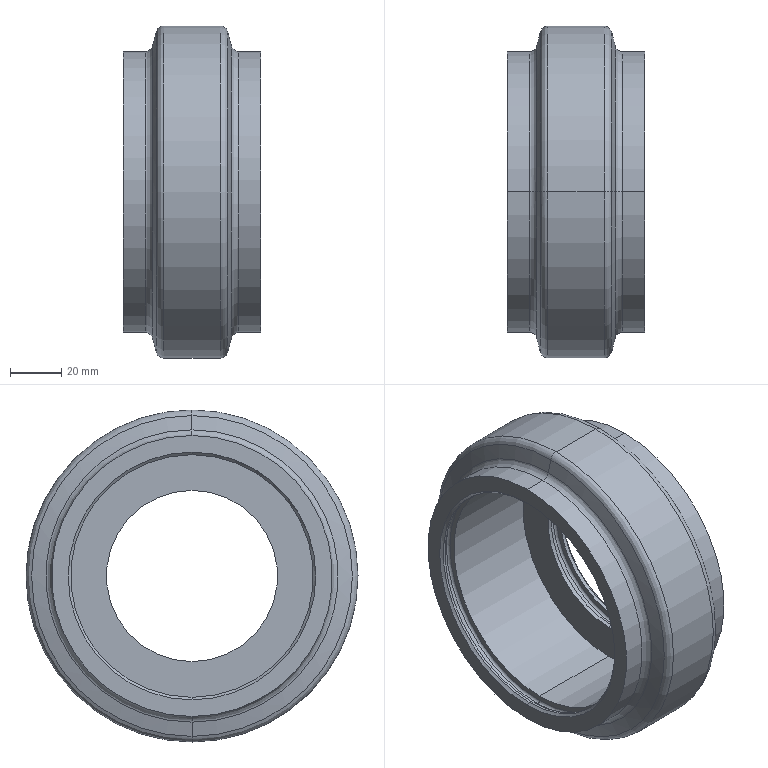Part | SolidWorks | features Chamfer 1, Revolution 1 | 1 solid | 49 faces | box 54 x 130 x 130 mm | volume 264733 mm3 | cylinder 18 | torus 16 | cone 8 | plane 7 | commonest cylinder face diameters 67 x4 95 x4 110 x4 73.2 x2 101.2 x2 130 x2
STEP:
#1=CARTESIAN_POINT('',(-26.,0.,-47.5));
#2=VERTEX_POINT('',#1);
#3=CARTESIAN_POINT('',(-26.,0.,47.5));
#4=VERTEX_POINT('',#3);
#5=CARTESIAN_POINT('',(-26.,0.,0.));
#6=DIRECTION('',(-1.,0.,0.));
#7=DIRECTION('',(0.,0.,1.));
#8=AXIS2_PLACEMENT_3D('',#5,#6,#7);
#9=CIRCLE('',#8,47.5);
#10=EDGE_CURVE('',#2,#4,#9,.T.);
#11=ORIENTED_EDGE('',*,*,#10,.F.);
#12=CARTESIAN_POINT('',(-27.,0.,-48.5));
#13=VERTEX_POINT('',#12);
#14=CARTESIAN_POINT('',(-27.,0.,-48.5));
#15=DIRECTION('',(-0.7071,0.,-0.7071));
#16=VECTOR('',#15,1000.);
#17=LINE('',#14,#16);
#18=EDGE_CURVE('',#2,#13,#17,.T.);
#19=ORIENTED_EDGE('',*,*,#18,.T.);
#20=CARTESIAN_POINT('',(-27.,0.,48.5));
#21=VERTEX_POINT('',#20);
#22=CARTESIAN_POINT('',(-27.,0.,0.));
#23=DIRECTION('',(1.,0.,0.));
#24=DIRECTION('',(0.,0.,1.));
#25=AXIS2_PLACEMENT_3D('',#22,#23,#24);
#26=CIRCLE('',#25,48.5);
#27=EDGE_CURVE('',#21,#13,#26,.T.);
#28=ORIENTED_EDGE('',*,*,#27,.F.);
#29=CARTESIAN_POINT('',(-27.,0.,48.5));
#30=DIRECTION('',(-0.7071,0.,0.7071));
#31=VECTOR('',#30,1000.);
#32=LINE('',#29,#31);
#33=EDGE_CURVE('',#4,#21,#32,.T.);
#34=ORIENTED_EDGE('',*,*,#33,.F.);
#35=EDGE_LOOP('',(#11,#19,#28,#34));
#36=FACE_OUTER_BOUND('',#35,.T.);
#37=CARTESIAN_POINT('',(-27.,0.,0.));
#38=DIRECTION('',(-1.,0.,0.));
#39=DIRECTION('',(0.,0.,1.));
#40=AXIS2_PLACEMENT_3D('',#37,#38,#39);
#41=CONICAL_SURFACE('',#40,48.5,0.7854);
#42=ADVANCED_FACE('',(#36),#41,.F.);
#43=CARTESIAN_POINT('',(26.,0.,33.5));
#44=VERTEX_POINT('',#43);
#45=CARTESIAN_POINT('',(26.,0.,-33.5));
#46=VERTEX_POINT('',#45);
#47=CARTESIAN_POINT('',(26.,0.,0.));
#48=DIRECTION('',(1.,0.,0.));
#49=DIRECTION('',(0.,0.,-1.));
#50=AXIS2_PLACEMENT_3D('',#47,#48,#49);
#51=CIRCLE('',#50,33.5);
#52=EDGE_CURVE('',#44,#46,#51,.T.);
#53=ORIENTED_EDGE('',*,*,#52,.F.);
#54=CARTESIAN_POINT('',(27.,0.,34.5));
#55=VERTEX_POINT('',#54);
#56=CARTESIAN_POINT('',(26.,0.,33.5));
#57=DIRECTION('',(0.7071,0.,0.7071));
#58=VECTOR('',#57,1000.);
#59=LINE('',#56,#58);
#60=EDGE_CURVE('',#44,#55,#59,.T.);
#61=ORIENTED_EDGE('',*,*,#60,.T.);
#62=CARTESIAN_POINT('',(27.,0.,-34.5));
#63=VERTEX_POINT('',#62);
#64=CARTESIAN_POINT('',(27.,0.,0.));
#65=DIRECTION('',(-1.,0.,0.));
#66=DIRECTION('',(0.,0.,-1.));
#67=AXIS2_PLACEMENT_3D('',#64,#65,#66);
#68=CIRCLE('',#67,34.5);
#69=EDGE_CURVE('',#63,#55,#68,.T.);
#70=ORIENTED_EDGE('',*,*,#69,.F.);
#71=CARTESIAN_POINT('',(26.,0.,-33.5));
#72=DIRECTION('',(0.7071,0.,-0.7071));
#73=VECTOR('',#72,1000.);
#74=LINE('',#71,#73);
#75=EDGE_CURVE('',#46,#63,#74,.T.);
#76=ORIENTED_EDGE('',*,*,#75,.F.);
#77=EDGE_LOOP('',(#53,#61,#70,#76));
#78=FACE_OUTER_BOUND('',#77,.T.);
#79=CARTESIAN_POINT('',(26.,0.,0.));
#80=DIRECTION('',(1.,0.,0.));
#81=DIRECTION('',(0.,0.,-1.));
#82=AXIS2_PLACEMENT_3D('',#79,#80,#81);
#83=CONICAL_SURFACE('',#82,33.5,0.7854);
#84=ADVANCED_FACE('',(#78),#83,.F.);
#85=ORIENTED_EDGE('',*,*,#10,.T.);
#86=CARTESIAN_POINT('',(-25.,0.,47.5));
#87=VERTEX_POINT('',#86);
#88=CARTESIAN_POINT('',(27.,0.,47.5));
#89=DIRECTION('',(1.,0.,0.));
#90=VECTOR('',#89,1000.);
#91=LINE('',#88,#90);
#92=EDGE_CURVE('',#4,#87,#91,.T.);
#93=ORIENTED_EDGE('',*,*,#92,.T.);
#94=CARTESIAN_POINT('',(-25.,0.,-47.5));
#95=VERTEX_POINT('',#94);
#96=CARTESIAN_POINT('',(-25.,0.,0.));
#97=DIRECTION('',(1.,0.,0.));
#98=DIRECTION('',(0.,0.,-1.));
#99=AXIS2_PLACEMENT_3D('',#96,#97,#98);
#100=CIRCLE('',#99,47.5);
#101=EDGE_CURVE('',#87,#95,#100,.T.);
#102=ORIENTED_EDGE('',*,*,#101,.T.);
#103=CARTESIAN_POINT('',(27.,0.,-47.5));
#104=DIRECTION('',(1.,0.,0.));
#105=VECTOR('',#104,1000.);
#106=LINE('',#103,#105);
#107=EDGE_CURVE('',#2,#95,#106,.T.);
#108=ORIENTED_EDGE('',*,*,#107,.F.);
#109=EDGE_LOOP('',(#85,#93,#102,#108));
#110=FACE_OUTER_BOUND('',#109,.T.);
#111=CARTESIAN_POINT('',(27.,0.,0.));
#112=DIRECTION('',(1.,0.,0.));
#113=DIRECTION('',(0.,0.,-1.));
#114=AXIS2_PLACEMENT_3D('',#111,#112,#113);
#115=CYLINDRICAL_SURFACE('',#114,47.5);
#116=ADVANCED_FACE('',(#110),#115,.F.);
#117=CARTESIAN_POINT('',(-25.,0.,49.6));
#118=VERTEX_POINT('',#117);
#119=CARTESIAN_POINT('',(-25.,0.,-49.6));
#120=VERTEX_POINT('',#119);
#121=CARTESIAN_POINT('',(-25.,0.,0.));
#122=DIRECTION('',(1.,0.,0.));
#123=DIRECTION('',(0.,0.,-1.));
#124=AXIS2_PLACEMENT_3D('',#121,#122,#123);
#125=CIRCLE('',#124,49.6);
#126=EDGE_CURVE('',#118,#120,#125,.T.);
#127=ORIENTED_EDGE('',*,*,#126,.F.);
#128=CARTESIAN_POINT('',(-24.,0.,50.6));
#129=VERTEX_POINT('',#128);
#130=CARTESIAN_POINT('',(-24.,0.,49.6));
#131=DIRECTION('',(0.,1.,0.));
#132=DIRECTION('',(0.,0.,1.));
#133=AXIS2_PLACEMENT_3D('',#130,#131,#132);
#134=CIRCLE('',#133,1.);
#135=EDGE_CURVE('',#118,#129,#134,.T.);
#136=ORIENTED_EDGE('',*,*,#135,.T.);
#137=CARTESIAN_POINT('',(-24.,0.,-50.6));
#138=VERTEX_POINT('',#137);
#139=CARTESIAN_POINT('',(-24.,0.,0.));
#140=DIRECTION('',(1.,0.,0.));
#141=DIRECTION('',(0.,0.,-1.));
#142=AXIS2_PLACEMENT_3D('',#139,#140,#141);
#143=CIRCLE('',#142,50.6);
#144=EDGE_CURVE('',#129,#138,#143,.T.);
#145=ORIENTED_EDGE('',*,*,#144,.T.);
#146=CARTESIAN_POINT('',(-24.,0.,-49.6));
#147=DIRECTION('',(0.,-1.,0.));
#148=DIRECTION('',(0.,0.,-1.));
#149=AXIS2_PLACEMENT_3D('',#146,#147,#148);
#150=CIRCLE('',#149,1.);
#151=EDGE_CURVE('',#120,#138,#150,.T.);
#152=ORIENTED_EDGE('',*,*,#151,.F.);
#153=EDGE_LOOP('',(#127,#136,#145,#152));
#154=FACE_OUTER_BOUND('',#153,.T.);
#155=CARTESIAN_POINT('',(-24.,0.,0.));
#156=DIRECTION('',(1.,0.,0.));
#157=DIRECTION('',(0.,0.,-1.));
#158=AXIS2_PLACEMENT_3D('',#155,#156,#157);
#159=TOROIDAL_SURFACE('',#158,49.6,1.);
#160=ADVANCED_FACE('',(#154),#159,.F.);
#161=ORIENTED_EDGE('',*,*,#144,.F.);
#162=CARTESIAN_POINT('',(-21.2,0.,50.6));
#163=VERTEX_POINT('',#162);
#164=CARTESIAN_POINT('',(27.,0.,50.6));
#165=DIRECTION('',(1.,0.,0.));
#166=VECTOR('',#165,1000.);
#167=LINE('',#164,#166);
#168=EDGE_CURVE('',#129,#163,#167,.T.);
#169=ORIENTED_EDGE('',*,*,#168,.T.);
#170=CARTESIAN_POINT('',(-21.2,0.,-50.6));
#171=VERTEX_POINT('',#170);
#172=CARTESIAN_POINT('',(-21.2,0.,0.));
#173=DIRECTION('',(1.,0.,0.));
#174=DIRECTION('',(0.,0.,-1.));
#175=AXIS2_PLACEMENT_3D('',#172,#173,#174);
#176=CIRCLE('',#175,50.6);
#177=EDGE_CURVE('',#163,#171,#176,.T.);
#178=ORIENTED_EDGE('',*,*,#177,.T.);
#179=CARTESIAN_POINT('',(27.,0.,-50.6));
#180=DIRECTION('',(1.,0.,0.));
#181=VECTOR('',#180,1000.);
#182=LINE('',#179,#181);
#183=EDGE_CURVE('',#138,#171,#182,.T.);
#184=ORIENTED_EDGE('',*,*,#183,.F.);
#185=EDGE_LOOP('',(#161,#169,#178,#184));
#186=FACE_OUTER_BOUND('',#185,.T.);
#187=CARTESIAN_POINT('',(27.,0.,0.));
#188=DIRECTION('',(1.,0.,0.));
#189=DIRECTION('',(0.,0.,-1.));
#190=AXIS2_PLACEMENT_3D('',#187,#188,#189);
#191=CYLINDRICAL_SURFACE('',#190,50.6);
#192=ADVANCED_FACE('',(#186),#191,.F.);
#193=ORIENTED_EDGE('',*,*,#177,.F.);
#194=CARTESIAN_POINT('',(-20.2,0.,49.6));
#195=VERTEX_POINT('',#194);
#196=CARTESIAN_POINT('',(-21.2,0.,49.6));
#197=DIRECTION('',(0.,1.,0.));
#198=DIRECTION('',(0.,0.,1.));
#199=AXIS2_PLACEMENT_3D('',#196,#197,#198);
#200=CIRCLE('',#199,1.);
#201=EDGE_CURVE('',#163,#195,#200,.T.);
#202=ORIENTED_EDGE('',*,*,#201,.T.);
#203=CARTESIAN_POINT('',(-20.2,0.,-49.6));
#204=VERTEX_POINT('',#203);
#205=CARTESIAN_POINT('',(-20.2,0.,0.));
#206=DIRECTION('',(1.,0.,0.));
#207=DIRECTION('',(0.,0.,-1.));
#208=AXIS2_PLACEMENT_3D('',#205,#206,#207);
#209=CIRCLE('',#208,49.6);
#210=EDGE_CURVE('',#195,#204,#209,.T.);
#211=ORIENTED_EDGE('',*,*,#210,.T.);
#212=CARTESIAN_POINT('',(-21.2,0.,-49.6));
#213=DIRECTION('',(0.,-1.,0.));
#214=DIRECTION('',(0.,0.,-1.));
#215=AXIS2_PLACEMENT_3D('',#212,#213,#214);
#216=CIRCLE('',#215,1.);
#217=EDGE_CURVE('',#171,#204,#216,.T.);
#218=ORIENTED_EDGE('',*,*,#217,.F.);
#219=EDGE_LOOP('',(#193,#202,#211,#218));
#220=FACE_OUTER_BOUND('',#219,.T.);
#221=CARTESIAN_POINT('',(-21.2,0.,0.));
#222=DIRECTION('',(1.,0.,0.));
#223=DIRECTION('',(0.,0.,-1.));
#224=AXIS2_PLACEMENT_3D('',#221,#222,#223);
#225=TOROIDAL_SURFACE('',#224,49.6,1.);
#226=ADVANCED_FACE('',(#220),#225,.F.);
#227=CARTESIAN_POINT('',(-20.2,0.,47.5));
#228=VERTEX_POINT('',#227);
#229=CARTESIAN_POINT('',(-20.2,0.,-47.5));
#230=VERTEX_POINT('',#229);
#231=CARTESIAN_POINT('',(-20.2,0.,0.));
#232=DIRECTION('',(1.,0.,0.));
#233=DIRECTION('',(0.,0.,-1.));
#234=AXIS2_PLACEMENT_3D('',#231,#232,#233);
#235=CIRCLE('',#234,47.5);
#236=EDGE_CURVE('',#228,#230,#235,.T.);
#237=ORIENTED_EDGE('',*,*,#236,.F.);
#238=CARTESIAN_POINT('',(18.,0.,47.5));
#239=VERTEX_POINT('',#238);
#240=CARTESIAN_POINT('',(27.,0.,47.5));
#241=DIRECTION('',(1.,0.,0.));
#242=VECTOR('',#241,1000.);
#243=LINE('',#240,#242);
#244=EDGE_CURVE('',#228,#239,#243,.T.);
#245=ORIENTED_EDGE('',*,*,#244,.T.);
#246=CARTESIAN_POINT('',(18.,0.,-47.5));
#247=VERTEX_POINT('',#246);
#248=CARTESIAN_POINT('',(18.,0.,0.));
#249=DIRECTION('',(1.,0.,0.));
#250=DIRECTION('',(0.,0.,-1.));
#251=AXIS2_PLACEMENT_3D('',#248,#249,#250);
#252=CIRCLE('',#251,47.5);
#253=EDGE_CURVE('',#239,#247,#252,.T.);
#254=ORIENTED_EDGE('',*,*,#253,.T.);
#255=CARTESIAN_POINT('',(27.,0.,-47.5));
#256=DIRECTION('',(1.,0.,0.));
#257=VECTOR('',#256,1000.);
#258=LINE('',#255,#257);
#259=EDGE_CURVE('',#230,#247,#258,.T.);
#260=ORIENTED_EDGE('',*,*,#259,.F.);
#261=EDGE_LOOP('',(#237,#245,#254,#260));
#262=FACE_OUTER_BOUND('',#261,.T.);
#263=CARTESIAN_POINT('',(27.,0.,0.));
#264=DIRECTION('',(1.,0.,0.));
#265=DIRECTION('',(0.,0.,-1.));
#266=AXIS2_PLACEMENT_3D('',#263,#264,#265);
#267=CYLINDRICAL_SURFACE('',#266,47.5);
#268=ADVANCED_FACE('',(#262),#267,.F.);
#269=CARTESIAN_POINT('',(18.,0.,33.5));
#270=VERTEX_POINT('',#269);
#271=CARTESIAN_POINT('',(18.,0.,-33.5));
#272=VERTEX_POINT('',#271);
#273=CARTESIAN_POINT('',(18.,0.,0.));
#274=DIRECTION('',(1.,0.,0.));
#275=DIRECTION('',(0.,0.,-1.));
#276=AXIS2_PLACEMENT_3D('',#273,#274,#275);
#277=CIRCLE('',#276,33.5);
#278=EDGE_CURVE('',#270,#272,#277,.T.);
#279=ORIENTED_EDGE('',*,*,#278,.F.);
#280=CARTESIAN_POINT('',(19.7,0.,33.5));
#281=VERTEX_POINT('',#280);
#282=CARTESIAN_POINT('',(27.,0.,33.5));
#283=DIRECTION('',(1.,0.,0.));
#284=VECTOR('',#283,1000.);
#285=LINE('',#282,#284);
#286=EDGE_CURVE('',#270,#281,#285,.T.);
#287=ORIENTED_EDGE('',*,*,#286,.T.);
#288=CARTESIAN_POINT('',(19.7,0.,-33.5));
#289=VERTEX_POINT('',#288);
#290=CARTESIAN_POINT('',(19.7,0.,0.));
#291=DIRECTION('',(1.,0.,0.));
#292=DIRECTION('',(0.,0.,-1.));
#293=AXIS2_PLACEMENT_3D('',#290,#291,#292);
#294=CIRCLE('',#293,33.5);
#295=EDGE_CURVE('',#281,#289,#294,.T.);
#296=ORIENTED_EDGE('',*,*,#295,.T.);
#297=CARTESIAN_POINT('',(27.,0.,-33.5));
#298=DIRECTION('',(1.,0.,0.));
#299=VECTOR('',#298,1000.);
#300=LINE('',#297,#299);
#301=EDGE_CURVE('',#272,#289,#300,.T.);
#302=ORIENTED_EDGE('',*,*,#301,.F.);
#303=EDGE_LOOP('',(#279,#287,#296,#302));
#304=FACE_OUTER_BOUND('',#303,.T.);
#305=CARTESIAN_POINT('',(27.,0.,0.));
#306=DIRECTION('',(1.,0.,0.));
#307=DIRECTION('',(0.,0.,-1.));
#308=AXIS2_PLACEMENT_3D('',#305,#306,#307);
#309=CYLINDRICAL_SURFACE('',#308,33.5);
#310=ADVANCED_FACE('',(#304),#309,.F.);
#311=CARTESIAN_POINT('',(19.7,0.,35.6));
#312=VERTEX_POINT('',#311);
#313=CARTESIAN_POINT('',(19.7,0.,-35.6));
#314=VERTEX_POINT('',#313);
#315=CARTESIAN_POINT('',(19.7,0.,0.));
#316=DIRECTION('',(1.,0.,0.));
#317=DIRECTION('',(0.,0.,-1.));
#318=AXIS2_PLACEMENT_3D('',#315,#316,#317);
#319=CIRCLE('',#318,35.6);
#320=EDGE_CURVE('',#312,#314,#319,.T.);
#321=ORIENTED_EDGE('',*,*,#320,.F.);
#322=CARTESIAN_POINT('',(20.7,0.,36.6));
#323=VERTEX_POINT('',#322);
#324=CARTESIAN_POINT('',(20.7,0.,35.6));
#325=DIRECTION('',(0.,1.,0.));
#326=DIRECTION('',(0.,0.,1.));
#327=AXIS2_PLACEMENT_3D('',#324,#325,#326);
#328=CIRCLE('',#327,1.);
#329=EDGE_CURVE('',#312,#323,#328,.T.);
#330=ORIENTED_EDGE('',*,*,#329,.T.);
#331=CARTESIAN_POINT('',(20.7,0.,-36.6));
#332=VERTEX_POINT('',#331);
#333=CARTESIAN_POINT('',(20.7,0.,0.));
#334=DIRECTION('',(1.,0.,0.));
#335=DIRECTION('',(0.,0.,-1.));
#336=AXIS2_PLACEMENT_3D('',#333,#334,#335);
#337=CIRCLE('',#336,36.6);
#338=EDGE_CURVE('',#323,#332,#337,.T.);
#339=ORIENTED_EDGE('',*,*,#338,.T.);
#340=CARTESIAN_POINT('',(20.7,0.,-35.6));
#341=DIRECTION('',(0.,-1.,0.));
#342=DIRECTION('',(0.,0.,-1.));
#343=AXIS2_PLACEMENT_3D('',#340,#341,#342);
#344=CIRCLE('',#343,1.);
#345=EDGE_CURVE('',#314,#332,#344,.T.);
#346=ORIENTED_EDGE('',*,*,#345,.F.);
#347=EDGE_LOOP('',(#321,#330,#339,#346));
#348=FACE_OUTER_BOUND('',#347,.T.);
#349=CARTESIAN_POINT('',(20.7,0.,0.));
#350=DIRECTION('',(1.,0.,0.));
#351=DIRECTION('',(0.,0.,-1.));
#352=AXIS2_PLACEMENT_3D('',#349,#350,#351);
#353=TOROIDAL_SURFACE('',#352,35.6,1.);
#354=ADVANCED_FACE('',(#348),#353,.F.);
#355=ORIENTED_EDGE('',*,*,#338,.F.);
#356=CARTESIAN_POINT('',(23.5,0.,36.6));
#357=VERTEX_POINT('',#356);
#358=CARTESIAN_POINT('',(27.,0.,36.6));
#359=DIRECTION('',(1.,0.,0.));
#360=VECTOR('',#359,1000.);
#361=LINE('',#358,#360);
#362=EDGE_CURVE('',#323,#357,#361,.T.);
#363=ORIENTED_EDGE('',*,*,#362,.T.);
#364=CARTESIAN_POINT('',(23.5,0.,-36.6));
#365=VERTEX_POINT('',#364);
#366=CARTESIAN_POINT('',(23.5,0.,0.));
#367=DIRECTION('',(1.,0.,0.));
#368=DIRECTION('',(0.,0.,-1.));
#369=AXIS2_PLACEMENT_3D('',#366,#367,#368);
#370=CIRCLE('',#369,36.6);
#371=EDGE_CURVE('',#357,#365,#370,.T.);
#372=ORIENTED_EDGE('',*,*,#371,.T.);
#373=CARTESIAN_POINT('',(27.,0.,-36.6));
#374=DIRECTION('',(1.,0.,0.));
#375=VECTOR('',#374,1000.);
#376=LINE('',#373,#375);
#377=EDGE_CURVE('',#332,#365,#376,.T.);
#378=ORIENTED_EDGE('',*,*,#377,.F.);
#379=EDGE_LOOP('',(#355,#363,#372,#378));
#380=FACE_OUTER_BOUND('',#379,.T.);
#381=CARTESIAN_POINT('',(27.,0.,0.));
#382=DIRECTION('',(1.,0.,0.));
#383=DIRECTION('',(0.,0.,-1.));
#384=AXIS2_PLACEMENT_3D('',#381,#382,#383);
#385=CYLINDRICAL_SURFACE('',#384,36.6);
#386=ADVANCED_FACE('',(#380),#385,.F.);
#387=ORIENTED_EDGE('',*,*,#371,.F.);
#388=CARTESIAN_POINT('',(24.5,0.,35.6));
#389=VERTEX_POINT('',#388);
#390=CARTESIAN_POINT('',(23.5,0.,35.6));
#391=DIRECTION('',(0.,1.,0.));
#392=DIRECTION('',(0.,0.,1.));
#393=AXIS2_PLACEMENT_3D('',#390,#391,#392);
#394=CIRCLE('',#393,1.);
#395=EDGE_CURVE('',#357,#389,#394,.T.);
#396=ORIENTED_EDGE('',*,*,#395,.T.);
#397=CARTESIAN_POINT('',(24.5,0.,-35.6));
#398=VERTEX_POINT('',#397);
#399=CARTESIAN_POINT('',(24.5,0.,0.));
#400=DIRECTION('',(1.,0.,0.));
#401=DIRECTION('',(0.,0.,-1.));
#402=AXIS2_PLACEMENT_3D('',#399,#400,#401);
#403=CIRCLE('',#402,35.6);
#404=EDGE_CURVE('',#389,#398,#403,.T.);
#405=ORIENTED_EDGE('',*,*,#404,.T.);
#406=CARTESIAN_POINT('',(23.5,0.,-35.6));
#407=DIRECTION('',(0.,-1.,0.));
#408=DIRECTION('',(0.,0.,-1.));
#409=AXIS2_PLACEMENT_3D('',#406,#407,#408);
#410=CIRCLE('',#409,1.);
#411=EDGE_CURVE('',#365,#398,#410,.T.);
#412=ORIENTED_EDGE('',*,*,#411,.F.);
#413=EDGE_LOOP('',(#387,#396,#405,#412));
#414=FACE_OUTER_BOUND('',#413,.T.);
#415=CARTESIAN_POINT('',(23.5,0.,0.));
#416=DIRECTION('',(1.,0.,0.));
#417=DIRECTION('',(0.,0.,-1.));
#418=AXIS2_PLACEMENT_3D('',#415,#416,#417);
#419=TOROIDAL_SURFACE('',#418,35.6,1.);
#420=ADVANCED_FACE('',(#414),#419,.F.);
#421=CARTESIAN_POINT('',(24.5,0.,33.5));
#422=VERTEX_POINT('',#421);
#423=CARTESIAN_POINT('',(24.5,0.,-33.5));
#424=VERTEX_POINT('',#423);
#425=CARTESIAN_POINT('',(24.5,0.,0.));
#426=DIRECTION('',(1.,0.,0.));
#427=DIRECTION('',(0.,0.,-1.));
#428=AXIS2_PLACEMENT_3D('',#425,#426,#427);
#429=CIRCLE('',#428,33.5);
#430=EDGE_CURVE('',#422,#424,#429,.T.);
#431=ORIENTED_EDGE('',*,*,#430,.F.);
#432=CARTESIAN_POINT('',(27.,0.,33.5));
#433=DIRECTION('',(1.,0.,0.));
#434=VECTOR('',#433,1000.);
#435=LINE('',#432,#434);
#436=EDGE_CURVE('',#422,#44,#435,.T.);
#437=ORIENTED_EDGE('',*,*,#436,.T.);
#438=ORIENTED_EDGE('',*,*,#52,.T.);
#439=CARTESIAN_POINT('',(27.,0.,-33.5));
#440=DIRECTION('',(1.,0.,0.));
#441=VECTOR('',#440,1000.);
#442=LINE('',#439,#441);
#443=EDGE_CURVE('',#424,#46,#442,.T.);
#444=ORIENTED_EDGE('',*,*,#443,.F.);
#445=EDGE_LOOP('',(#431,#437,#438,#444));
#446=FACE_OUTER_BOUND('',#445,.T.);
#447=CARTESIAN_POINT('',(27.,0.,0.));
#448=DIRECTION('',(1.,0.,0.));
#449=DIRECTION('',(0.,0.,-1.));
#450=AXIS2_PLACEMENT_3D('',#447,#448,#449);
#451=CYLINDRICAL_SURFACE('',#450,33.5);
#452=ADVANCED_FACE('',(#446),#451,.F.);
#453=CARTESIAN_POINT('',(18.302,0.,-55.));
#454=VERTEX_POINT('',#453);
#455=CARTESIAN_POINT('',(18.302,0.,55.));
#456=VERTEX_POINT('',#455);
#457=CARTESIAN_POINT('',(18.302,0.,0.));
#458=DIRECTION('',(1.,0.,0.));
#459=DIRECTION('',(0.,0.,-1.));
#460=AXIS2_PLACEMENT_3D('',#457,#458,#459);
#461=CIRCLE('',#460,55.);
#462=EDGE_CURVE('',#454,#456,#461,.T.);
#463=ORIENTED_EDGE('',*,*,#462,.T.);
#464=CARTESIAN_POINT('',(27.,0.,55.));
#465=VERTEX_POINT('',#464);
#466=CARTESIAN_POINT('',(27.,0.,55.));
#467=DIRECTION('',(1.,0.,0.));
#468=VECTOR('',#467,1000.);
#469=LINE('',#466,#468);
#470=EDGE_CURVE('',#456,#465,#469,.T.);
#471=ORIENTED_EDGE('',*,*,#470,.T.);
#472=CARTESIAN_POINT('',(27.,0.,-55.));
#473=VERTEX_POINT('',#472);
#474=CARTESIAN_POINT('',(27.,0.,0.));
#475=DIRECTION('',(1.,0.,0.));
#476=DIRECTION('',(0.,0.,-1.));
#477=AXIS2_PLACEMENT_3D('',#474,#475,#476);
#478=CIRCLE('',#477,55.);
#479=EDGE_CURVE('',#473,#465,#478,.T.);
#480=ORIENTED_EDGE('',*,*,#479,.F.);
#481=CARTESIAN_POINT('',(27.,0.,-55.));
#482=DIRECTION('',(1.,0.,0.));
#483=VECTOR('',#482,1000.);
#484=LINE('',#481,#483);
#485=EDGE_CURVE('',#454,#473,#484,.T.);
#486=ORIENTED_EDGE('',*,*,#485,.F.);
#487=EDGE_LOOP('',(#463,#471,#480,#486));
#488=FACE_OUTER_BOUND('',#487,.T.);
#489=CARTESIAN_POINT('',(27.,0.,0.));
#490=DIRECTION('',(1.,0.,0.));
#491=DIRECTION('',(0.,0.,-1.));
#492=AXIS2_PLACEMENT_3D('',#489,#490,#491);
#493=CYLINDRICAL_SURFACE('',#492,55.);
#494=ADVANCED_FACE('',(#488),#493,.T.);
#495=CARTESIAN_POINT('',(18.302,0.,0.));
#496=DIRECTION('',(1.,0.,0.));
#497=DIRECTION('',(0.,0.,-1.));
#498=AXIS2_PLACEMENT_3D('',#495,#496,#497);
#499=CIRCLE('',#498,55.);
#500=EDGE_CURVE('',#456,#454,#499,.T.);
#501=ORIENTED_EDGE('',*,*,#500,.F.);
#502=CARTESIAN_POINT('',(15.404,0.,57.224));
#503=VERTEX_POINT('',#502);
#504=CARTESIAN_POINT('',(18.302,0.,58.));
#505=DIRECTION('',(0.,1.,0.));
#506=DIRECTION('',(0.,0.,1.));
#507=AXIS2_PLACEMENT_3D('',#504,#505,#506);
#508=CIRCLE('',#507,3.);
#509=EDGE_CURVE('',#456,#503,#508,.T.);
#510=ORIENTED_EDGE('',*,*,#509,.T.);
#511=CARTESIAN_POINT('',(15.404,0.,-57.224));
#512=VERTEX_POINT('',#511);
#513=CARTESIAN_POINT('',(15.404,0.,0.));
#514=DIRECTION('',(1.,0.,0.));
#515=DIRECTION('',(0.,0.,-1.));
#516=AXIS2_PLACEMENT_3D('',#513,#514,#515);
#517=CIRCLE('',#516,57.224);
#518=EDGE_CURVE('',#503,#512,#517,.T.);
#519=ORIENTED_EDGE('',*,*,#518,.T.);
#520=CARTESIAN_POINT('',(18.302,0.,-58.));
#521=DIRECTION('',(0.,-1.,0.));
#522=DIRECTION('',(0.,0.,-1.));
#523=AXIS2_PLACEMENT_3D('',#520,#521,#522);
#524=CIRCLE('',#523,3.);
#525=EDGE_CURVE('',#454,#512,#524,.T.);
#526=ORIENTED_EDGE('',*,*,#525,.F.);
#527=EDGE_LOOP('',(#501,#510,#519,#526));
#528=FACE_OUTER_BOUND('',#527,.T.);
#529=CARTESIAN_POINT('',(18.302,0.,0.));
#530=DIRECTION('',(1.,0.,0.));
#531=DIRECTION('',(0.,0.,-1.));
#532=AXIS2_PLACEMENT_3D('',#529,#530,#531);
#533=TOROIDAL_SURFACE('',#532,58.,3.);
#534=ADVANCED_FACE('',(#528),#533,.F.);
#535=CARTESIAN_POINT('',(15.404,0.,0.));
#536=DIRECTION('',(1.,0.,0.));
#537=DIRECTION('',(0.,0.,-1.));
#538=AXIS2_PLACEMENT_3D('',#535,#536,#537);
#539=CIRCLE('',#538,57.224);
#540=EDGE_CURVE('',#512,#503,#539,.T.);
#541=ORIENTED_EDGE('',*,*,#540,.F.);
#542=CARTESIAN_POINT('',(13.916,0.,-62.776));
#543=VERTEX_POINT('',#542);
#544=CARTESIAN_POINT('',(15.404,0.,-57.224));
#545=DIRECTION('',(-0.2588,0.,-0.9659));
#546=VECTOR('',#545,1000.);
#547=LINE('',#544,#546);
#548=EDGE_CURVE('',#512,#543,#547,.T.);
#549=ORIENTED_EDGE('',*,*,#548,.T.);
#550=CARTESIAN_POINT('',(13.916,0.,62.776));
#551=VERTEX_POINT('',#550);
#552=CARTESIAN_POINT('',(13.916,0.,0.));
#553=DIRECTION('',(1.,0.,0.));
#554=DIRECTION('',(0.,0.,-1.));
#555=AXIS2_PLACEMENT_3D('',#552,#553,#554);
#556=CIRCLE('',#555,62.776);
#557=EDGE_CURVE('',#543,#551,#556,.T.);
#558=ORIENTED_EDGE('',*,*,#557,.T.);
#559=CARTESIAN_POINT('',(15.404,0.,57.224));
#560=DIRECTION('',(-0.2588,0.,0.9659));
#561=VECTOR('',#560,1000.);
#562=LINE('',#559,#561);
#563=EDGE_CURVE('',#503,#551,#562,.T.);
#564=ORIENTED_EDGE('',*,*,#563,.F.);
#565=EDGE_LOOP('',(#541,#549,#558,#564));
#566=FACE_OUTER_BOUND('',#565,.T.);
#567=CARTESIAN_POINT('',(15.404,0.,0.));
#568=DIRECTION('',(-1.,0.,0.));
#569=DIRECTION('',(0.,0.,1.));
#570=AXIS2_PLACEMENT_3D('',#567,#568,#569);
#571=CONICAL_SURFACE('',#570,57.224,1.309);
#572=ADVANCED_FACE('',(#566),#571,.T.);
#573=CARTESIAN_POINT('',(11.019,0.,-65.));
#574=VERTEX_POINT('',#573);
#575=CARTESIAN_POINT('',(11.019,0.,65.));
#576=VERTEX_POINT('',#575);
#577=CARTESIAN_POINT('',(11.019,0.,0.));
#578=DIRECTION('',(1.,0.,0.));
#579=DIRECTION('',(0.,0.,-1.));
#580=AXIS2_PLACEMENT_3D('',#577,#578,#579);
#581=CIRCLE('',#580,65.);
#582=EDGE_CURVE('',#574,#576,#581,.T.);
#583=ORIENTED_EDGE('',*,*,#582,.T.);
#584=CARTESIAN_POINT('',(11.019,0.,62.));
#585=DIRECTION('',(0.,1.,0.));
#586=DIRECTION('',(0.,0.,1.));
#587=AXIS2_PLACEMENT_3D('',#584,#585,#586);
#588=CIRCLE('',#587,3.);
#589=EDGE_CURVE('',#576,#551,#588,.T.);
#590=ORIENTED_EDGE('',*,*,#589,.T.);
#591=ORIENTED_EDGE('',*,*,#557,.F.);
#592=CARTESIAN_POINT('',(11.019,0.,-62.));
#593=DIRECTION('',(0.,-1.,0.));
#594=DIRECTION('',(0.,0.,-1.));
#595=AXIS2_PLACEMENT_3D('',#592,#593,#594);
#596=CIRCLE('',#595,3.);
#597=EDGE_CURVE('',#574,#543,#596,.T.);
#598=ORIENTED_EDGE('',*,*,#597,.F.);
#599=EDGE_LOOP('',(#583,#590,#591,#598));
#600=FACE_OUTER_BOUND('',#599,.T.);
#601=CARTESIAN_POINT('',(11.019,0.,0.));
#602=DIRECTION('',(1.,0.,0.));
#603=DIRECTION('',(0.,0.,-1.));
#604=AXIS2_PLACEMENT_3D('',#601,#602,#603);
#605=TOROIDAL_SURFACE('',#604,62.,3.);
#606=ADVANCED_FACE('',(#600),#605,.T.);
#607=CARTESIAN_POINT('',(-11.019,0.,-65.));
#608=VERTEX_POINT('',#607);
#609=CARTESIAN_POINT('',(-11.019,0.,65.));
#610=VERTEX_POINT('',#609);
#611=CARTESIAN_POINT('',(-11.019,0.,0.));
#612=DIRECTION('',(1.,0.,0.));
#613=DIRECTION('',(0.,0.,-1.));
#614=AXIS2_PLACEMENT_3D('',#611,#612,#613);
#615=CIRCLE('',#614,65.);
#616=EDGE_CURVE('',#608,#610,#615,.T.);
#617=ORIENTED_EDGE('',*,*,#616,.T.);
#618=CARTESIAN_POINT('',(27.,0.,65.));
#619=DIRECTION('',(1.,0.,0.));
#620=VECTOR('',#619,1000.);
#621=LINE('',#618,#620);
#622=EDGE_CURVE('',#610,#576,#621,.T.);
#623=ORIENTED_EDGE('',*,*,#622,.T.);
#624=ORIENTED_EDGE('',*,*,#582,.F.);
#625=CARTESIAN_POINT('',(27.,0.,-65.));
#626=DIRECTION('',(1.,0.,0.));
#627=VECTOR('',#626,1000.);
#628=LINE('',#625,#627);
#629=EDGE_CURVE('',#608,#574,#628,.T.);
#630=ORIENTED_EDGE('',*,*,#629,.F.);
#631=EDGE_LOOP('',(#617,#623,#624,#630));
#632=FACE_OUTER_BOUND('',#631,.T.);
#633=CARTESIAN_POINT('',(27.,0.,0.));
#634=DIRECTION('',(1.,0.,0.));
#635=DIRECTION('',(0.,0.,-1.));
#636=AXIS2_PLACEMENT_3D('',#633,#634,#635);
#637=CYLINDRICAL_SURFACE('',#636,65.);
#638=ADVANCED_FACE('',(#632),#637,.T.);
#639=CARTESIAN_POINT('',(-13.916,0.,-62.776));
#640=VERTEX_POINT('',#639);
#641=CARTESIAN_POINT('',(-13.916,0.,62.776));
#642=VERTEX_POINT('',#641);
#643=CARTESIAN_POINT('',(-13.916,0.,0.));
#644=DIRECTION('',(1.,0.,0.));
#645=DIRECTION('',(0.,0.,-1.));
#646=AXIS2_PLACEMENT_3D('',#643,#644,#645);
#647=CIRCLE('',#646,62.776);
#648=EDGE_CURVE('',#640,#642,#647,.T.);
#649=ORIENTED_EDGE('',*,*,#648,.T.);
#650=CARTESIAN_POINT('',(-11.019,0.,62.));
#651=DIRECTION('',(0.,1.,0.));
#652=DIRECTION('',(0.,0.,1.));
#653=AXIS2_PLACEMENT_3D('',#650,#651,#652);
#654=CIRCLE('',#653,3.);
#655=EDGE_CURVE('',#642,#610,#654,.T.);
#656=ORIENTED_EDGE('',*,*,#655,.T.);
#657=ORIENTED_EDGE('',*,*,#616,.F.);
#658=CARTESIAN_POINT('',(-11.019,0.,-62.));
#659=DIRECTION('',(0.,-1.,0.));
#660=DIRECTION('',(0.,0.,-1.));
#661=AXIS2_PLACEMENT_3D('',#658,#659,#660);
#662=CIRCLE('',#661,3.);
#663=EDGE_CURVE('',#640,#608,#662,.T.);
#664=ORIENTED_EDGE('',*,*,#663,.F.);
#665=EDGE_LOOP('',(#649,#656,#657,#664));
#666=FACE_OUTER_BOUND('',#665,.T.);
#667=CARTESIAN_POINT('',(-11.019,0.,0.));
#668=DIRECTION('',(1.,0.,0.));
#669=DIRECTION('',(0.,0.,-1.));
#670=AXIS2_PLACEMENT_3D('',#667,#668,#669);
#671=TOROIDAL_SURFACE('',#670,62.,3.);
#672=ADVANCED_FACE('',(#666),#671,.T.);
#673=CARTESIAN_POINT('',(-15.404,0.,-57.224));
#674=VERTEX_POINT('',#673);
#675=CARTESIAN_POINT('',(-15.404,0.,57.224));
#676=VERTEX_POINT('',#675);
#677=CARTESIAN_POINT('',(-15.404,0.,0.));
#678=DIRECTION('',(1.,0.,0.));
#679=DIRECTION('',(0.,0.,-1.));
#680=AXIS2_PLACEMENT_3D('',#677,#678,#679);
#681=CIRCLE('',#680,57.224);
#682=EDGE_CURVE('',#674,#676,#681,.T.);
#683=ORIENTED_EDGE('',*,*,#682,.T.);
#684=CARTESIAN_POINT('',(-13.916,0.,62.776));
#685=DIRECTION('',(0.2588,0.,0.9659));
#686=VECTOR('',#685,1000.);
#687=LINE('',#684,#686);
#688=EDGE_CURVE('',#676,#642,#687,.T.);
#689=ORIENTED_EDGE('',*,*,#688,.T.);
#690=ORIENTED_EDGE('',*,*,#648,.F.);
#691=CARTESIAN_POINT('',(-13.916,0.,-62.776));
#692=DIRECTION('',(0.2588,0.,-0.9659));
#693=VECTOR('',#692,1000.);
#694=LINE('',#691,#693);
#695=EDGE_CURVE('',#674,#640,#694,.T.);
#696=ORIENTED_EDGE('',*,*,#695,.F.);
#697=EDGE_LOOP('',(#683,#689,#690,#696));
#698=FACE_OUTER_BOUND('',#697,.T.);
#699=CARTESIAN_POINT('',(-13.916,0.,0.));
#700=DIRECTION('',(1.,0.,0.));
#701=DIRECTION('',(0.,0.,-1.));
#702=AXIS2_PLACEMENT_3D('',#699,#700,#701);
#703=CONICAL_SURFACE('',#702,62.776,1.309);
#704=ADVANCED_FACE('',(#698),#703,.T.);
#705=CARTESIAN_POINT('',(-15.404,0.,0.));
#706=DIRECTION('',(1.,0.,0.));
#707=DIRECTION('',(0.,0.,-1.));
#708=AXIS2_PLACEMENT_3D('',#705,#706,#707);
#709=CIRCLE('',#708,57.224);
#710=EDGE_CURVE('',#676,#674,#709,.T.);
#711=ORIENTED_EDGE('',*,*,#710,.F.);
#712=CARTESIAN_POINT('',(-18.302,0.,55.));
#713=VERTEX_POINT('',#712);
#714=CARTESIAN_POINT('',(-18.302,0.,58.));
#715=DIRECTION('',(0.,1.,0.));
#716=DIRECTION('',(0.,0.,1.));
#717=AXIS2_PLACEMENT_3D('',#714,#715,#716);
#718=CIRCLE('',#717,3.);
#719=EDGE_CURVE('',#676,#713,#718,.T.);
#720=ORIENTED_EDGE('',*,*,#719,.T.);
#721=CARTESIAN_POINT('',(-18.302,0.,-55.));
#722=VERTEX_POINT('',#721);
#723=CARTESIAN_POINT('',(-18.302,0.,0.));
#724=DIRECTION('',(1.,0.,0.));
#725=DIRECTION('',(0.,0.,-1.));
#726=AXIS2_PLACEMENT_3D('',#723,#724,#725);
#727=CIRCLE('',#726,55.);
#728=EDGE_CURVE('',#713,#722,#727,.T.);
#729=ORIENTED_EDGE('',*,*,#728,.T.);
#730=CARTESIAN_POINT('',(-18.302,0.,-58.));
#731=DIRECTION('',(0.,-1.,0.));
#732=DIRECTION('',(0.,0.,-1.));
#733=AXIS2_PLACEMENT_3D('',#730,#731,#732);
#734=CIRCLE('',#733,3.);
#735=EDGE_CURVE('',#674,#722,#734,.T.);
#736=ORIENTED_EDGE('',*,*,#735,.F.);
#737=EDGE_LOOP('',(#711,#720,#729,#736));
#738=FACE_OUTER_BOUND('',#737,.T.);
#739=CARTESIAN_POINT('',(-18.302,0.,0.));
#740=DIRECTION('',(1.,0.,0.));
#741=DIRECTION('',(0.,0.,-1.));
#742=AXIS2_PLACEMENT_3D('',#739,#740,#741);
#743=TOROIDAL_SURFACE('',#742,58.,3.);
#744=ADVANCED_FACE('',(#738),#743,.F.);
#745=CARTESIAN_POINT('',(-27.,0.,-55.));
#746=VERTEX_POINT('',#745);
#747=CARTESIAN_POINT('',(-27.,0.,55.));
#748=VERTEX_POINT('',#747);
#749=CARTESIAN_POINT('',(-27.,0.,0.));
#750=DIRECTION('',(1.,0.,0.));
#751=DIRECTION('',(0.,0.,-1.));
#752=AXIS2_PLACEMENT_3D('',#749,#750,#751);
#753=CIRCLE('',#752,55.);
#754=EDGE_CURVE('',#746,#748,#753,.T.);
#755=ORIENTED_EDGE('',*,*,#754,.T.);
#756=CARTESIAN_POINT('',(27.,0.,55.));
#757=DIRECTION('',(1.,0.,0.));
#758=VECTOR('',#757,1000.);
#759=LINE('',#756,#758);
#760=EDGE_CURVE('',#748,#713,#759,.T.);
#761=ORIENTED_EDGE('',*,*,#760,.T.);
#762=CARTESIAN_POINT('',(-18.302,0.,0.));
#763=DIRECTION('',(1.,0.,0.));
#764=DIRECTION('',(0.,0.,-1.));
#765=AXIS2_PLACEMENT_3D('',#762,#763,#764);
#766=CIRCLE('',#765,55.);
#767=EDGE_CURVE('',#722,#713,#766,.T.);
#768=ORIENTED_EDGE('',*,*,#767,.F.);
#769=CARTESIAN_POINT('',(27.,0.,-55.));
#770=DIRECTION('',(1.,0.,0.));
#771=VECTOR('',#770,1000.);
#772=LINE('',#769,#771);
#773=EDGE_CURVE('',#746,#722,#772,.T.);
#774=ORIENTED_EDGE('',*,*,#773,.F.);
#775=EDGE_LOOP('',(#755,#761,#768,#774));
#776=FACE_OUTER_BOUND('',#775,.T.);
#777=CARTESIAN_POINT('',(27.,0.,0.));
#778=DIRECTION('',(1.,0.,0.));
#779=DIRECTION('',(0.,0.,-1.));
#780=AXIS2_PLACEMENT_3D('',#777,#778,#779);
#781=CYLINDRICAL_SURFACE('',#780,55.);
#782=ADVANCED_FACE('',(#776),#781,.T.);
#783=ORIENTED_EDGE('',*,*,#760,.F.);
#784=CARTESIAN_POINT('',(-27.,0.,0.));
#785=DIRECTION('',(1.,0.,0.));
#786=DIRECTION('',(0.,0.,-1.));
#787=AXIS2_PLACEMENT_3D('',#784,#785,#786);
#788=CIRCLE('',#787,55.);
#789=EDGE_CURVE('',#748,#746,#788,.T.);
#790=ORIENTED_EDGE('',*,*,#789,.T.);
#791=ORIENTED_EDGE('',*,*,#773,.T.);
#792=ORIENTED_EDGE('',*,*,#728,.F.);
#793=EDGE_LOOP('',(#783,#790,#791,#792));
#794=FACE_OUTER_BOUND('',#793,.T.);
#795=CARTESIAN_POINT('',(27.,0.,0.));
#796=DIRECTION('',(1.,0.,0.));
#797=DIRECTION('',(0.,0.,-1.));
#798=AXIS2_PLACEMENT_3D('',#795,#796,#797);
#799=CYLINDRICAL_SURFACE('',#798,55.);
#800=ADVANCED_FACE('',(#794),#799,.T.);
#801=ORIENTED_EDGE('',*,*,#719,.F.);
#802=ORIENTED_EDGE('',*,*,#682,.F.);
#803=ORIENTED_EDGE('',*,*,#735,.T.);
#804=ORIENTED_EDGE('',*,*,#767,.T.);
#805=EDGE_LOOP('',(#801,#802,#803,#804));
#806=FACE_OUTER_BOUND('',#805,.T.);
#807=CARTESIAN_POINT('',(-18.302,0.,0.));
#808=DIRECTION('',(1.,0.,0.));
#809=DIRECTION('',(0.,0.,-1.));
#810=AXIS2_PLACEMENT_3D('',#807,#808,#809);
#811=TOROIDAL_SURFACE('',#810,58.,3.);
#812=ADVANCED_FACE('',(#806),#811,.F.);
#813=ORIENTED_EDGE('',*,*,#688,.F.);
#814=ORIENTED_EDGE('',*,*,#710,.T.);
#815=ORIENTED_EDGE('',*,*,#695,.T.);
#816=CARTESIAN_POINT('',(-13.916,0.,0.));
#817=DIRECTION('',(1.,0.,0.));
#818=DIRECTION('',(0.,0.,-1.));
#819=AXIS2_PLACEMENT_3D('',#816,#817,#818);
#820=CIRCLE('',#819,62.776);
#821=EDGE_CURVE('',#642,#640,#820,.T.);
#822=ORIENTED_EDGE('',*,*,#821,.F.);
#823=EDGE_LOOP('',(#813,#814,#815,#822));
#824=FACE_OUTER_BOUND('',#823,.T.);
#825=CARTESIAN_POINT('',(-13.916,0.,0.));
#826=DIRECTION('',(1.,0.,0.));
#827=DIRECTION('',(0.,0.,-1.));
#828=AXIS2_PLACEMENT_3D('',#825,#826,#827);
#829=CONICAL_SURFACE('',#828,62.776,1.309);
#830=ADVANCED_FACE('',(#824),#829,.T.);
#831=ORIENTED_EDGE('',*,*,#655,.F.);
#832=ORIENTED_EDGE('',*,*,#821,.T.);
#833=ORIENTED_EDGE('',*,*,#663,.T.);
#834=CARTESIAN_POINT('',(-11.019,0.,0.));
#835=DIRECTION('',(1.,0.,0.));
#836=DIRECTION('',(0.,0.,-1.));
#837=AXIS2_PLACEMENT_3D('',#834,#835,#836);
#838=CIRCLE('',#837,65.);
#839=EDGE_CURVE('',#610,#608,#838,.T.);
#840=ORIENTED_EDGE('',*,*,#839,.F.);
#841=EDGE_LOOP('',(#831,#832,#833,#840));
#842=FACE_OUTER_BOUND('',#841,.T.);
#843=CARTESIAN_POINT('',(-11.019,0.,0.));
#844=DIRECTION('',(1.,0.,0.));
#845=DIRECTION('',(0.,0.,-1.));
#846=AXIS2_PLACEMENT_3D('',#843,#844,#845);
#847=TOROIDAL_SURFACE('',#846,62.,3.);
#848=ADVANCED_FACE('',(#842),#847,.T.);
#849=ORIENTED_EDGE('',*,*,#622,.F.);
#850=ORIENTED_EDGE('',*,*,#839,.T.);
#851=ORIENTED_EDGE('',*,*,#629,.T.);
#852=CARTESIAN_POINT('',(11.019,0.,0.));
#853=DIRECTION('',(1.,0.,0.));
#854=DIRECTION('',(0.,0.,-1.));
#855=AXIS2_PLACEMENT_3D('',#852,#853,#854);
#856=CIRCLE('',#855,65.);
#857=EDGE_CURVE('',#576,#574,#856,.T.);
#858=ORIENTED_EDGE('',*,*,#857,.F.);
#859=EDGE_LOOP('',(#849,#850,#851,#858));
#860=FACE_OUTER_BOUND('',#859,.T.);
#861=CARTESIAN_POINT('',(27.,0.,0.));
#862=DIRECTION('',(1.,0.,0.));
#863=DIRECTION('',(0.,0.,-1.));
#864=AXIS2_PLACEMENT_3D('',#861,#862,#863);
#865=CYLINDRICAL_SURFACE('',#864,65.);
#866=ADVANCED_FACE('',(#860),#865,.T.);
#867=ORIENTED_EDGE('',*,*,#589,.F.);
#868=ORIENTED_EDGE('',*,*,#857,.T.);
#869=ORIENTED_EDGE('',*,*,#597,.T.);
#870=CARTESIAN_POINT('',(13.916,0.,0.));
#871=DIRECTION('',(1.,0.,0.));
#872=DIRECTION('',(0.,0.,-1.));
#873=AXIS2_PLACEMENT_3D('',#870,#871,#872);
#874=CIRCLE('',#873,62.776);
#875=EDGE_CURVE('',#551,#543,#874,.T.);
#876=ORIENTED_EDGE('',*,*,#875,.F.);
#877=EDGE_LOOP('',(#867,#868,#869,#876));
#878=FACE_OUTER_BOUND('',#877,.T.);
#879=CARTESIAN_POINT('',(11.019,0.,0.));
#880=DIRECTION('',(1.,0.,0.));
#881=DIRECTION('',(0.,0.,-1.));
#882=AXIS2_PLACEMENT_3D('',#879,#880,#881);
#883=TOROIDAL_SURFACE('',#882,62.,3.);
#884=ADVANCED_FACE('',(#878),#883,.T.);
#885=ORIENTED_EDGE('',*,*,#548,.F.);
#886=ORIENTED_EDGE('',*,*,#518,.F.);
#887=ORIENTED_EDGE('',*,*,#563,.T.);
#888=ORIENTED_EDGE('',*,*,#875,.T.);
#889=EDGE_LOOP('',(#885,#886,#887,#888));
#890=FACE_OUTER_BOUND('',#889,.T.);
#891=CARTESIAN_POINT('',(15.404,0.,0.));
#892=DIRECTION('',(-1.,0.,0.));
#893=DIRECTION('',(0.,0.,1.));
#894=AXIS2_PLACEMENT_3D('',#891,#892,#893);
#895=CONICAL_SURFACE('',#894,57.224,1.309);
#896=ADVANCED_FACE('',(#890),#895,.T.);
#897=ORIENTED_EDGE('',*,*,#509,.F.);
#898=ORIENTED_EDGE('',*,*,#462,.F.);
#899=ORIENTED_EDGE('',*,*,#525,.T.);
#900=ORIENTED_EDGE('',*,*,#540,.T.);
#901=EDGE_LOOP('',(#897,#898,#899,#900));
#902=FACE_OUTER_BOUND('',#901,.T.);
#903=CARTESIAN_POINT('',(18.302,0.,0.));
#904=DIRECTION('',(1.,0.,0.));
#905=DIRECTION('',(0.,0.,-1.));
#906=AXIS2_PLACEMENT_3D('',#903,#904,#905);
#907=TOROIDAL_SURFACE('',#906,58.,3.);
#908=ADVANCED_FACE('',(#902),#907,.F.);
#909=ORIENTED_EDGE('',*,*,#470,.F.);
#910=ORIENTED_EDGE('',*,*,#500,.T.);
#911=ORIENTED_EDGE('',*,*,#485,.T.);
#912=CARTESIAN_POINT('',(27.,0.,0.));
#913=DIRECTION('',(1.,0.,0.));
#914=DIRECTION('',(0.,0.,-1.));
#915=AXIS2_PLACEMENT_3D('',#912,#913,#914);
#916=CIRCLE('',#915,55.);
#917=EDGE_CURVE('',#465,#473,#916,.T.);
#918=ORIENTED_EDGE('',*,*,#917,.F.);
#919=EDGE_LOOP('',(#909,#910,#911,#918));
#920=FACE_OUTER_BOUND('',#919,.T.);
#921=CARTESIAN_POINT('',(27.,0.,0.));
#922=DIRECTION('',(1.,0.,0.));
#923=DIRECTION('',(0.,0.,-1.));
#924=AXIS2_PLACEMENT_3D('',#921,#922,#923);
#925=CYLINDRICAL_SURFACE('',#924,55.);
#926=ADVANCED_FACE('',(#920),#925,.T.);
#927=ORIENTED_EDGE('',*,*,#69,.T.);
#928=CARTESIAN_POINT('',(27.,0.,0.));
#929=DIRECTION('',(-1.,0.,0.));
#930=DIRECTION('',(0.,0.,-1.));
#931=AXIS2_PLACEMENT_3D('',#928,#929,#930);
#932=CIRCLE('',#931,34.5);
#933=EDGE_CURVE('',#55,#63,#932,.T.);
#934=ORIENTED_EDGE('',*,*,#933,.T.);
#935=EDGE_LOOP('',(#927,#934));
#936=FACE_BOUND('',#935,.T.);
#937=ORIENTED_EDGE('',*,*,#479,.T.);
#938=ORIENTED_EDGE('',*,*,#917,.T.);
#939=EDGE_LOOP('',(#937,#938));
#940=FACE_OUTER_BOUND('',#939,.T.);
#941=CARTESIAN_POINT('',(27.,55.,0.));
#942=DIRECTION('',(1.,0.,0.));
#943=DIRECTION('',(0.,0.,-1.));
#944=AXIS2_PLACEMENT_3D('',#941,#942,#943);
#945=PLANE('',#944);
#946=ADVANCED_FACE('',(#936,#940),#945,.T.);
#947=ORIENTED_EDGE('',*,*,#436,.F.);
#948=CARTESIAN_POINT('',(24.5,0.,0.));
#949=DIRECTION('',(1.,0.,0.));
#950=DIRECTION('',(0.,0.,-1.));
#951=AXIS2_PLACEMENT_3D('',#948,#949,#950);
#952=CIRCLE('',#951,33.5);
#953=EDGE_CURVE('',#424,#422,#952,.T.);
#954=ORIENTED_EDGE('',*,*,#953,.F.);
#955=ORIENTED_EDGE('',*,*,#443,.T.);
#956=CARTESIAN_POINT('',(26.,0.,0.));
#957=DIRECTION('',(1.,0.,0.));
#958=DIRECTION('',(0.,0.,-1.));
#959=AXIS2_PLACEMENT_3D('',#956,#957,#958);
#960=CIRCLE('',#959,33.5);
#961=EDGE_CURVE('',#46,#44,#960,.T.);
#962=ORIENTED_EDGE('',*,*,#961,.T.);
#963=EDGE_LOOP('',(#947,#954,#955,#962));
#964=FACE_OUTER_BOUND('',#963,.T.);
#965=CARTESIAN_POINT('',(27.,0.,0.));
#966=DIRECTION('',(1.,0.,0.));
#967=DIRECTION('',(0.,0.,-1.));
#968=AXIS2_PLACEMENT_3D('',#965,#966,#967);
#969=CYLINDRICAL_SURFACE('',#968,33.5);
#970=ADVANCED_FACE('',(#964),#969,.F.);
#971=ORIENTED_EDGE('',*,*,#953,.T.);
#972=ORIENTED_EDGE('',*,*,#430,.T.);
#973=EDGE_LOOP('',(#971,#972));
#974=FACE_BOUND('',#973,.T.);
#975=CARTESIAN_POINT('',(24.5,0.,0.));
#976=DIRECTION('',(1.,0.,0.));
#977=DIRECTION('',(0.,0.,-1.));
#978=AXIS2_PLACEMENT_3D('',#975,#976,#977);
#979=CIRCLE('',#978,35.6);
#980=EDGE_CURVE('',#398,#389,#979,.T.);
#981=ORIENTED_EDGE('',*,*,#980,.F.);
#982=ORIENTED_EDGE('',*,*,#404,.F.);
#983=EDGE_LOOP('',(#981,#982));
#984=FACE_OUTER_BOUND('',#983,.T.);
#985=CARTESIAN_POINT('',(24.5,35.6,0.));
#986=DIRECTION('',(-1.,0.,0.));
#987=DIRECTION('',(0.,0.,1.));
#988=AXIS2_PLACEMENT_3D('',#985,#986,#987);
#989=PLANE('',#988);
#990=ADVANCED_FACE('',(#974,#984),#989,.T.);
#991=ORIENTED_EDGE('',*,*,#395,.F.);
#992=CARTESIAN_POINT('',(23.5,0.,0.));
#993=DIRECTION('',(1.,0.,0.));
#994=DIRECTION('',(0.,0.,-1.));
#995=AXIS2_PLACEMENT_3D('',#992,#993,#994);
#996=CIRCLE('',#995,36.6);
#997=EDGE_CURVE('',#365,#357,#996,.T.);
#998=ORIENTED_EDGE('',*,*,#997,.F.);
#999=ORIENTED_EDGE('',*,*,#411,.T.);
#1000=ORIENTED_EDGE('',*,*,#980,.T.);
#1001=EDGE_LOOP('',(#991,#998,#999,#1000));
#1002=FACE_OUTER_BOUND('',#1001,.T.);
#1003=CARTESIAN_POINT('',(23.5,0.,0.));
#1004=DIRECTION('',(1.,0.,0.));
#1005=DIRECTION('',(0.,0.,-1.));
#1006=AXIS2_PLACEMENT_3D('',#1003,#1004,#1005);
#1007=TOROIDAL_SURFACE('',#1006,35.6,1.);
#1008=ADVANCED_FACE('',(#1002),#1007,.F.);
#1009=ORIENTED_EDGE('',*,*,#362,.F.);
#1010=CARTESIAN_POINT('',(20.7,0.,0.));
#1011=DIRECTION('',(1.,0.,0.));
#1012=DIRECTION('',(0.,0.,-1.));
#1013=AXIS2_PLACEMENT_3D('',#1010,#1011,#1012);
#1014=CIRCLE('',#1013,36.6);
#1015=EDGE_CURVE('',#332,#323,#1014,.T.);
#1016=ORIENTED_EDGE('',*,*,#1015,.F.);
#1017=ORIENTED_EDGE('',*,*,#377,.T.);
#1018=ORIENTED_EDGE('',*,*,#997,.T.);
#1019=EDGE_LOOP('',(#1009,#1016,#1017,#1018));
#1020=FACE_OUTER_BOUND('',#1019,.T.);
#1021=CARTESIAN_POINT('',(27.,0.,0.));
#1022=DIRECTION('',(1.,0.,0.));
#1023=DIRECTION('',(0.,0.,-1.));
#1024=AXIS2_PLACEMENT_3D('',#1021,#1022,#1023);
#1025=CYLINDRICAL_SURFACE('',#1024,36.6);
#1026=ADVANCED_FACE('',(#1020),#1025,.F.);
#1027=ORIENTED_EDGE('',*,*,#329,.F.);
#1028=CARTESIAN_POINT('',(19.7,0.,0.));
#1029=DIRECTION('',(1.,0.,0.));
#1030=DIRECTION('',(0.,0.,-1.));
#1031=AXIS2_PLACEMENT_3D('',#1028,#1029,#1030);
#1032=CIRCLE('',#1031,35.6);
#1033=EDGE_CURVE('',#314,#312,#1032,.T.);
#1034=ORIENTED_EDGE('',*,*,#1033,.F.);
#1035=ORIENTED_EDGE('',*,*,#345,.T.);
#1036=ORIENTED_EDGE('',*,*,#1015,.T.);
#1037=EDGE_LOOP('',(#1027,#1034,#1035,#1036));
#1038=FACE_OUTER_BOUND('',#1037,.T.);
#1039=CARTESIAN_POINT('',(20.7,0.,0.));
#1040=DIRECTION('',(1.,0.,0.));
#1041=DIRECTION('',(0.,0.,-1.));
#1042=AXIS2_PLACEMENT_3D('',#1039,#1040,#1041);
#1043=TOROIDAL_SURFACE('',#1042,35.6,1.);
#1044=ADVANCED_FACE('',(#1038),#1043,.F.);
#1045=ORIENTED_EDGE('',*,*,#1033,.T.);
#1046=ORIENTED_EDGE('',*,*,#320,.T.);
#1047=EDGE_LOOP('',(#1045,#1046));
#1048=FACE_OUTER_BOUND('',#1047,.T.);
#1049=CARTESIAN_POINT('',(19.7,0.,0.));
#1050=DIRECTION('',(1.,0.,0.));
#1051=DIRECTION('',(0.,0.,-1.));
#1052=AXIS2_PLACEMENT_3D('',#1049,#1050,#1051);
#1053=CIRCLE('',#1052,33.5);
#1054=EDGE_CURVE('',#289,#281,#1053,.T.);
#1055=ORIENTED_EDGE('',*,*,#1054,.F.);
#1056=ORIENTED_EDGE('',*,*,#295,.F.);
#1057=EDGE_LOOP('',(#1055,#1056));
#1058=FACE_BOUND('',#1057,.T.);
#1059=CARTESIAN_POINT('',(19.7,33.5,0.));
#1060=DIRECTION('',(1.,0.,0.));
#1061=DIRECTION('',(0.,0.,-1.));
#1062=AXIS2_PLACEMENT_3D('',#1059,#1060,#1061);
#1063=PLANE('',#1062);
#1064=ADVANCED_FACE('',(#1048,#1058),#1063,.T.);
#1065=ORIENTED_EDGE('',*,*,#286,.F.);
#1066=CARTESIAN_POINT('',(18.,0.,0.));
#1067=DIRECTION('',(1.,0.,0.));
#1068=DIRECTION('',(0.,0.,-1.));
#1069=AXIS2_PLACEMENT_3D('',#1066,#1067,#1068);
#1070=CIRCLE('',#1069,33.5);
#1071=EDGE_CURVE('',#272,#270,#1070,.T.);
#1072=ORIENTED_EDGE('',*,*,#1071,.F.);
#1073=ORIENTED_EDGE('',*,*,#301,.T.);
#1074=ORIENTED_EDGE('',*,*,#1054,.T.);
#1075=EDGE_LOOP('',(#1065,#1072,#1073,#1074));
#1076=FACE_OUTER_BOUND('',#1075,.T.);
#1077=CARTESIAN_POINT('',(27.,0.,0.));
#1078=DIRECTION('',(1.,0.,0.));
#1079=DIRECTION('',(0.,0.,-1.));
#1080=AXIS2_PLACEMENT_3D('',#1077,#1078,#1079);
#1081=CYLINDRICAL_SURFACE('',#1080,33.5);
#1082=ADVANCED_FACE('',(#1076),#1081,.F.);
#1083=ORIENTED_EDGE('',*,*,#1071,.T.);
#1084=ORIENTED_EDGE('',*,*,#278,.T.);
#1085=EDGE_LOOP('',(#1083,#1084));
#1086=FACE_BOUND('',#1085,.T.);
#1087=CARTESIAN_POINT('',(18.,0.,0.));
#1088=DIRECTION('',(1.,0.,0.));
#1089=DIRECTION('',(0.,0.,-1.));
#1090=AXIS2_PLACEMENT_3D('',#1087,#1088,#1089);
#1091=CIRCLE('',#1090,47.5);
#1092=EDGE_CURVE('',#247,#239,#1091,.T.);
#1093=ORIENTED_EDGE('',*,*,#1092,.F.);
#1094=ORIENTED_EDGE('',*,*,#253,.F.);
#1095=EDGE_LOOP('',(#1093,#1094));
#1096=FACE_OUTER_BOUND('',#1095,.T.);
#1097=CARTESIAN_POINT('',(18.,47.5,0.));
#1098=DIRECTION('',(-1.,0.,0.));
#1099=DIRECTION('',(0.,0.,1.));
#1100=AXIS2_PLACEMENT_3D('',#1097,#1098,#1099);
#1101=PLANE('',#1100);
#1102=ADVANCED_FACE('',(#1086,#1096),#1101,.T.);
#1103=ORIENTED_EDGE('',*,*,#244,.F.);
#1104=CARTESIAN_POINT('',(-20.2,0.,0.));
#1105=DIRECTION('',(1.,0.,0.));
#1106=DIRECTION('',(0.,0.,-1.));
#1107=AXIS2_PLACEMENT_3D('',#1104,#1105,#1106);
#1108=CIRCLE('',#1107,47.5);
#1109=EDGE_CURVE('',#230,#228,#1108,.T.);
#1110=ORIENTED_EDGE('',*,*,#1109,.F.);
#1111=ORIENTED_EDGE('',*,*,#259,.T.);
#1112=ORIENTED_EDGE('',*,*,#1092,.T.);
#1113=EDGE_LOOP('',(#1103,#1110,#1111,#1112));
#1114=FACE_OUTER_BOUND('',#1113,.T.);
#1115=CARTESIAN_POINT('',(27.,0.,0.));
#1116=DIRECTION('',(1.,0.,0.));
#1117=DIRECTION('',(0.,0.,-1.));
#1118=AXIS2_PLACEMENT_3D('',#1115,#1116,#1117);
#1119=CYLINDRICAL_SURFACE('',#1118,47.5);
#1120=ADVANCED_FACE('',(#1114),#1119,.F.);
#1121=ORIENTED_EDGE('',*,*,#1109,.T.);
#1122=ORIENTED_EDGE('',*,*,#236,.T.);
#1123=EDGE_LOOP('',(#1121,#1122));
#1124=FACE_BOUND('',#1123,.T.);
#1125=CARTESIAN_POINT('',(-20.2,0.,0.));
#1126=DIRECTION('',(1.,0.,0.));
#1127=DIRECTION('',(0.,0.,-1.));
#1128=AXIS2_PLACEMENT_3D('',#1125,#1126,#1127);
#1129=CIRCLE('',#1128,49.6);
#1130=EDGE_CURVE('',#204,#195,#1129,.T.);
#1131=ORIENTED_EDGE('',*,*,#1130,.F.);
#1132=ORIENTED_EDGE('',*,*,#210,.F.);
#1133=EDGE_LOOP('',(#1131,#1132));
#1134=FACE_OUTER_BOUND('',#1133,.T.);
#1135=CARTESIAN_POINT('',(-20.2,49.6,0.));
#1136=DIRECTION('',(-1.,0.,0.));
#1137=DIRECTION('',(0.,0.,1.));
#1138=AXIS2_PLACEMENT_3D('',#1135,#1136,#1137);
#1139=PLANE('',#1138);
#1140=ADVANCED_FACE('',(#1124,#1134),#1139,.T.);
#1141=ORIENTED_EDGE('',*,*,#201,.F.);
#1142=CARTESIAN_POINT('',(-21.2,0.,0.));
#1143=DIRECTION('',(1.,0.,0.));
#1144=DIRECTION('',(0.,0.,-1.));
#1145=AXIS2_PLACEMENT_3D('',#1142,#1143,#1144);
#1146=CIRCLE('',#1145,50.6);
#1147=EDGE_CURVE('',#171,#163,#1146,.T.);
#1148=ORIENTED_EDGE('',*,*,#1147,.F.);
#1149=ORIENTED_EDGE('',*,*,#217,.T.);
#1150=ORIENTED_EDGE('',*,*,#1130,.T.);
#1151=EDGE_LOOP('',(#1141,#1148,#1149,#1150));
#1152=FACE_OUTER_BOUND('',#1151,.T.);
#1153=CARTESIAN_POINT('',(-21.2,0.,0.));
#1154=DIRECTION('',(1.,0.,0.));
#1155=DIRECTION('',(0.,0.,-1.));
#1156=AXIS2_PLACEMENT_3D('',#1153,#1154,#1155);
#1157=TOROIDAL_SURFACE('',#1156,49.6,1.);
#1158=ADVANCED_FACE('',(#1152),#1157,.F.);
#1159=ORIENTED_EDGE('',*,*,#168,.F.);
#1160=CARTESIAN_POINT('',(-24.,0.,0.));
#1161=DIRECTION('',(1.,0.,0.));
#1162=DIRECTION('',(0.,0.,-1.));
#1163=AXIS2_PLACEMENT_3D('',#1160,#1161,#1162);
#1164=CIRCLE('',#1163,50.6);
#1165=EDGE_CURVE('',#138,#129,#1164,.T.);
#1166=ORIENTED_EDGE('',*,*,#1165,.F.);
#1167=ORIENTED_EDGE('',*,*,#183,.T.);
#1168=ORIENTED_EDGE('',*,*,#1147,.T.);
#1169=EDGE_LOOP('',(#1159,#1166,#1167,#1168));
#1170=FACE_OUTER_BOUND('',#1169,.T.);
#1171=CARTESIAN_POINT('',(27.,0.,0.));
#1172=DIRECTION('',(1.,0.,0.));
#1173=DIRECTION('',(0.,0.,-1.));
#1174=AXIS2_PLACEMENT_3D('',#1171,#1172,#1173);
#1175=CYLINDRICAL_SURFACE('',#1174,50.6);
#1176=ADVANCED_FACE('',(#1170),#1175,.F.);
#1177=ORIENTED_EDGE('',*,*,#135,.F.);
#1178=CARTESIAN_POINT('',(-25.,0.,0.));
#1179=DIRECTION('',(1.,0.,0.));
#1180=DIRECTION('',(0.,0.,-1.));
#1181=AXIS2_PLACEMENT_3D('',#1178,#1179,#1180);
#1182=CIRCLE('',#1181,49.6);
#1183=EDGE_CURVE('',#120,#118,#1182,.T.);
#1184=ORIENTED_EDGE('',*,*,#1183,.F.);
#1185=ORIENTED_EDGE('',*,*,#151,.T.);
#1186=ORIENTED_EDGE('',*,*,#1165,.T.);
#1187=EDGE_LOOP('',(#1177,#1184,#1185,#1186));
#1188=FACE_OUTER_BOUND('',#1187,.T.);
#1189=CARTESIAN_POINT('',(-24.,0.,0.));
#1190=DIRECTION('',(1.,0.,0.));
#1191=DIRECTION('',(0.,0.,-1.));
#1192=AXIS2_PLACEMENT_3D('',#1189,#1190,#1191);
#1193=TOROIDAL_SURFACE('',#1192,49.6,1.);
#1194=ADVANCED_FACE('',(#1188),#1193,.F.);
#1195=ORIENTED_EDGE('',*,*,#1183,.T.);
#1196=ORIENTED_EDGE('',*,*,#126,.T.);
#1197=EDGE_LOOP('',(#1195,#1196));
#1198=FACE_OUTER_BOUND('',#1197,.T.);
#1199=CARTESIAN_POINT('',(-25.,0.,0.));
#1200=DIRECTION('',(1.,0.,0.));
#1201=DIRECTION('',(0.,0.,-1.));
#1202=AXIS2_PLACEMENT_3D('',#1199,#1200,#1201);
#1203=CIRCLE('',#1202,47.5);
#1204=EDGE_CURVE('',#95,#87,#1203,.T.);
#1205=ORIENTED_EDGE('',*,*,#1204,.F.);
#1206=ORIENTED_EDGE('',*,*,#101,.F.);
#1207=EDGE_LOOP('',(#1205,#1206));
#1208=FACE_BOUND('',#1207,.T.);
#1209=CARTESIAN_POINT('',(-25.,47.5,0.));
#1210=DIRECTION('',(1.,0.,0.));
#1211=DIRECTION('',(0.,0.,-1.));
#1212=AXIS2_PLACEMENT_3D('',#1209,#1210,#1211);
#1213=PLANE('',#1212);
#1214=ADVANCED_FACE('',(#1198,#1208),#1213,.T.);
#1215=ORIENTED_EDGE('',*,*,#92,.F.);
#1216=CARTESIAN_POINT('',(-26.,0.,0.));
#1217=DIRECTION('',(-1.,0.,0.));
#1218=DIRECTION('',(0.,0.,1.));
#1219=AXIS2_PLACEMENT_3D('',#1216,#1217,#1218);
#1220=CIRCLE('',#1219,47.5);
#1221=EDGE_CURVE('',#4,#2,#1220,.T.);
#1222=ORIENTED_EDGE('',*,*,#1221,.T.);
#1223=ORIENTED_EDGE('',*,*,#107,.T.);
#1224=ORIENTED_EDGE('',*,*,#1204,.T.);
#1225=EDGE_LOOP('',(#1215,#1222,#1223,#1224));
#1226=FACE_OUTER_BOUND('',#1225,.T.);
#1227=CARTESIAN_POINT('',(27.,0.,0.));
#1228=DIRECTION('',(1.,0.,0.));
#1229=DIRECTION('',(0.,0.,-1.));
#1230=AXIS2_PLACEMENT_3D('',#1227,#1228,#1229);
#1231=CYLINDRICAL_SURFACE('',#1230,47.5);
#1232=ADVANCED_FACE('',(#1226),#1231,.F.);
#1233=ORIENTED_EDGE('',*,*,#27,.T.);
#1234=CARTESIAN_POINT('',(-27.,0.,0.));
#1235=DIRECTION('',(1.,0.,0.));
#1236=DIRECTION('',(0.,0.,1.));
#1237=AXIS2_PLACEMENT_3D('',#1234,#1235,#1236);
#1238=CIRCLE('',#1237,48.5);
#1239=EDGE_CURVE('',#13,#21,#1238,.T.);
#1240=ORIENTED_EDGE('',*,*,#1239,.T.);
#1241=EDGE_LOOP('',(#1233,#1240));
#1242=FACE_BOUND('',#1241,.T.);
#1243=ORIENTED_EDGE('',*,*,#754,.F.);
#1244=ORIENTED_EDGE('',*,*,#789,.F.);
#1245=EDGE_LOOP('',(#1243,#1244));
#1246=FACE_OUTER_BOUND('',#1245,.T.);
#1247=CARTESIAN_POINT('',(-27.,47.5,0.));
#1248=DIRECTION('',(-1.,0.,0.));
#1249=DIRECTION('',(0.,0.,1.));
#1250=AXIS2_PLACEMENT_3D('',#1247,#1248,#1249);
#1251=PLANE('',#1250);
#1252=ADVANCED_FACE('',(#1242,#1246),#1251,.T.);
#1253=ORIENTED_EDGE('',*,*,#60,.F.);
#1254=ORIENTED_EDGE('',*,*,#961,.F.);
#1255=ORIENTED_EDGE('',*,*,#75,.T.);
#1256=ORIENTED_EDGE('',*,*,#933,.F.);
#1257=EDGE_LOOP('',(#1253,#1254,#1255,#1256));
#1258=FACE_OUTER_BOUND('',#1257,.T.);
#1259=CARTESIAN_POINT('',(26.,0.,0.));
#1260=DIRECTION('',(1.,0.,0.));
#1261=DIRECTION('',(0.,0.,-1.));
#1262=AXIS2_PLACEMENT_3D('',#1259,#1260,#1261);
#1263=CONICAL_SURFACE('',#1262,33.5,0.7854);
#1264=ADVANCED_FACE('',(#1258),#1263,.F.);
#1265=ORIENTED_EDGE('',*,*,#18,.F.);
#1266=ORIENTED_EDGE('',*,*,#1221,.F.);
#1267=ORIENTED_EDGE('',*,*,#33,.T.);
#1268=ORIENTED_EDGE('',*,*,#1239,.F.);
#1269=EDGE_LOOP('',(#1265,#1266,#1267,#1268));
#1270=FACE_OUTER_BOUND('',#1269,.T.);
#1271=CARTESIAN_POINT('',(-27.,0.,0.));
#1272=DIRECTION('',(-1.,0.,0.));
#1273=DIRECTION('',(0.,0.,1.));
#1274=AXIS2_PLACEMENT_3D('',#1271,#1272,#1273);
#1275=CONICAL_SURFACE('',#1274,48.5,0.7854);
#1276=ADVANCED_FACE('',(#1270),#1275,.F.);
#1277=CLOSED_SHELL('',(#42,#84,#116,#160,#192,#226,#268,#310,#354,#386,#420,#452,#494,#534,#572,#606,#638,#672,#704,#744,#782,#800,#812,#830,#848,#866,#884,#896,#908,#926,#946,#970,#990,#1008,#1026,#1044,#1064,#1082,#1102,#1120,#1140,#1158,#1176,#1194,#1214,#1232,#1252,#1264,#1276));
#1278=MANIFOLD_SOLID_BREP('',#1277);
#1279=CARTESIAN_POINT('',(0.,0.,0.));
#1280=DIRECTION('',(0.,0.,1.));
#1281=DIRECTION('',(1.,0.,0.));
#1282=AXIS2_PLACEMENT_3D('',#1279,#1280,#1281);
#1283=(LENGTH_UNIT()NAMED_UNIT(*)SI_UNIT(.MILLI.,.METRE.));
#1284=UNCERTAINTY_MEASURE_WITH_UNIT(LENGTH_MEASURE(0.00001),#1283,'','');
#1285=(NAMED_UNIT(*)PLANE_ANGLE_UNIT()SI_UNIT($,.RADIAN.));
#1286=(NAMED_UNIT(*)SI_UNIT($,.STERADIAN.)SOLID_ANGLE_UNIT());
#1287=(GEOMETRIC_REPRESENTATION_CONTEXT(3)GLOBAL_UNCERTAINTY_ASSIGNED_CONTEXT((#1284))GLOBAL_UNIT_ASSIGNED_CONTEXT((#1283,#1285,#1286))REPRESENTATION_CONTEXT('',''));
#1288=ADVANCED_BREP_SHAPE_REPRESENTATION('',(#1278,#1282),#1287);